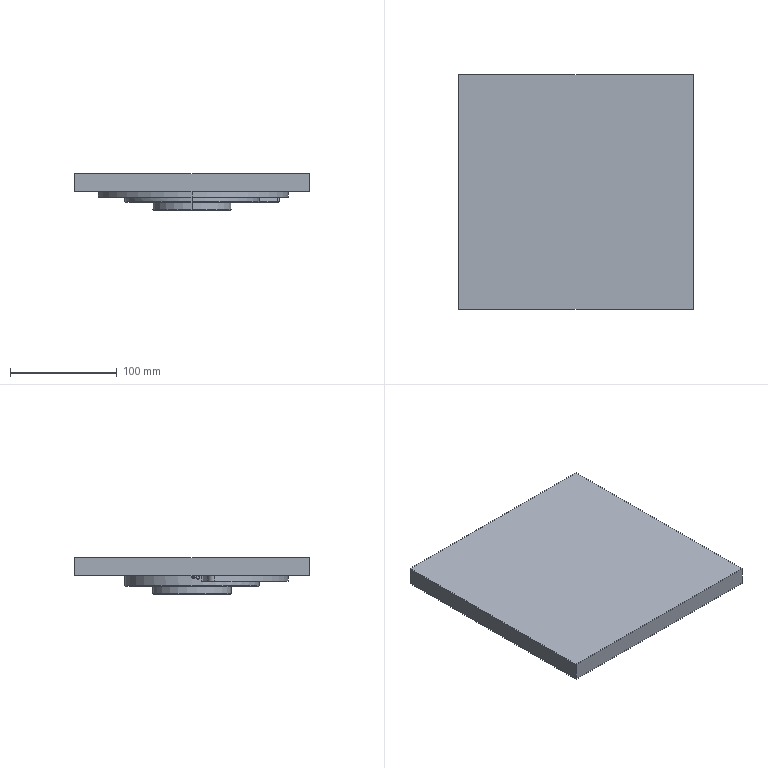NC program | NX | posted with a generic post | part box 220 x 220 x 34.5 mm
Lines 1 to 857 of 5610:
N10 G17 G21 G94 G90
(ADAPTIVE_MILLING_COPY_COPY , TOOL : D10)
N12 T03 M6
N14 G54
N16 G17 G0 G90 X77.604 Y4.579 S8000 M3
N18 G43 Z30. H3
N20 Z-4.5
N22 G94 G3 X77.604 Y4.579 Z-4.994 I3.735 J2.51 F1000.
N24 X77.604 Y4.579 Z-5.487 I3.735 J2.51
N26 X77.604 Y4.579 Z-5.981 I3.735 J2.51
N28 X77.604 Y4.579 Z-6.474 I3.735 J2.51
N30 X77.604 Y4.579 Z-6.968 I3.735 J2.51
N32 X77.604 Y4.579 Z-7.461 I3.735 J2.51
N34 X77.604 Y4.579 Z-7.955 I3.735 J2.51
N36 X77.604 Y4.579 Z-8.448 I3.735 J2.51
N38 X77.604 Y4.579 Z-8.942 I3.735 J2.51
N40 X77.604 Y4.579 Z-9.435 I3.735 J2.51
N42 X77.604 Y4.579 Z-9.929 I3.735 J2.51
N44 X77.604 Y4.579 Z-10.422 I3.735 J2.51
N46 X77.604 Y4.579 Z-10.916 I3.735 J2.51
N48 X77.604 Y4.579 Z-11.409 I3.735 J2.51
N50 X77.604 Y4.579 Z-11.903 I3.735 J2.51
N52 X76.839 Y7.09 Z-12.35 R-4.5
N54 X77.66 Y9.695 R-4.501 F3500.
N56 X82.637 Y2.294 R4.676
N58 X77.753 Y10.564 R-4.978
N60 X82.99 Y1.881 R5.196
N62 X77.662 Y11.175 R-5.477
N64 X83.422 Y1.484 R5.718
N66 X77.823 Y11.975 R-5.997
N68 X83.941 Y1.117 R6.258
N70 X77.688 Y12.541 R-6.537
N72 X84.559 Y0.793 R6.812
N74 X77.483 Y13.088 R-7.1
N76 X83.873 Y-0.126 R7.381
N78 X77.889 Y13.978 R-7.675
N80 X84.342 Y-0.592 R7.973
N82 X77.892 Y14.646 R-8.276
N84 X83.756 Y-1.428 R8.576
N86 X78.185 Y15.432 R-8.886
N88 X83.669 Y-2.101 R9.197
N90 X78.37 Y16.172 R-9.518
N92 X83.294 Y-2.846 R9.839
N94 X78.844 Y16.978 R-10.163
N96 X83.079 Y-3.549 R10.488
N98 X92.013 Y8.867 R10.816
N100 X79.62 Y17.804 R10.816
N102 X81.164 Y-4.346 R11.144
N104 X80.698 Y18.596 R-11.481
N106 X80.371 Y-4.984 R11.82
N108 X81.085 Y19.297 R-12.163
N110 X78.334 Y-5.339 R12.502
N112 X84.706 Y19.543 R12.843
N114 X69.985 Y0.098 R13.156
N116 X92.331 Y-0.932 R13.367
N118 X94.815 Y5.085 R13.688
N120 X94.218 Y11.135 R35.729
N122 X84.437 Y20.378 R13.14
N124 X67.552 Y8.958 R13.88
N126 X68.166 Y2.887 R147.626
N128 X74.962 Y-5.635 R12.919
N130 X94.942 Y2.514 R14.21
N132 G1 X94.812 Y5.136
N134 X94.408 Y10.154
N136 G3 X93.955 Y13.241 R19.214
N138 X89.674 Y18.793 R11.441
N140 X67.243 Y11.02 R14.568
N142 X67.535 Y9.129 R13.812
N144 G1 X67.56 Y8.88
N146 G3 X68.1 Y8.383 R0.554
N148 G1 X70.083 Y8.641 Z-12.25
N150 X91.724 Y11.521
N152 X93.706 Y11.786 Z-12.35
N154 G3 X94.152 Y12.389 R0.553
N156 X93.635 Y15.102 R9.567
N158 X88.948 Y20.151 R11.318
N160 X66.997 Y12.595 R15.277
N162 G1 X66.974 Y12.472
N164 X66.969 Y12.387
N166 X67.248 Y10.786
N168 G3 X67.828 Y10.331 R0.554
N170 G1 X69.813 Y10.576 Z-12.25
N172 X91.526 Y13.265
N174 X93.51 Y13.514 Z-12.35
N176 G3 X93.932 Y14.148 R0.553
N178 X93.286 Y16.681 R9.094
N180 X88.91 Y21.021 R10.806
N182 X66.842 Y14.109 R15.946
N184 G1 X66.796 Y13.993
N186 X66.757 Y13.874
N188 X66.741 Y13.75
N190 X66.739 Y13.708
N192 X66.975 Y12.354
N194 G3 X67.555 Y11.899 R0.554
N196 G1 X69.541 Y12.137 Z-12.25
N198 X91.273 Y14.75
N200 X93.258 Y14.993 Z-12.35
N202 G3 X93.665 Y15.624 R0.553
N204 X92.737 Y18.446 R6.65
N206 X87.147 Y22.693 R11.904
N208 X66.759 Y15.566 R16.65
N210 X66.653 Y14.203 R1.411
N212 G1 X66.76 Y13.587
N214 G3 X67.34 Y13.133 R0.554
N216 G1 X69.326 Y13.371 Z-12.25
N218 X91.05 Y15.98
N220 X93.035 Y16.223 Z-12.35
N222 G3 X93.442 Y16.854 R0.553
N224 X91.293 Y20.959 R6.144
N226 X82.546 Y24.546 R14.666
N228 X66.733 Y16.974 R17.347
N230 X66.254 Y15.782 R2.529
N232 G1 X66.53 Y14.691
N234 G3 X67.142 Y14.281 R0.554
N236 G1 X69.128 Y14.517 Z-12.25
N238 X90.851 Y17.091
N240 X92.836 Y17.33 Z-12.35
N242 G3 X93.242 Y17.962 R0.553
N244 X91.196 Y21.843 R5.78
N246 X83.037 Y25.286 R14.46
N248 X66.683 Y18.235 R17.99
N250 X66.01 Y16.748 R2.99
N252 G1 X66.255 Y15.778
N254 G3 X66.885 Y15.371 R0.555
N256 G1 X68.872 Y15.597 Z-12.25
N258 X90.672 Y18.083
N260 X92.658 Y18.314 Z-12.35
N262 G3 X93.064 Y18.946 R0.553
N264 X90.875 Y22.904 R5.754
N266 X82.991 Y26.077 R14.51
N268 X66.72 Y19.544 R18.632
N270 X65.767 Y17.806 R4.756
N272 G1 X65.769 Y17.698
N274 X66.015 Y16.728
N276 G3 X66.643 Y16.321 R0.555
N278 G1 X68.629 Y16.558 Z-12.25
N280 X90.475 Y19.167
N282 X92.46 Y19.41 Z-12.35
N284 G3 X92.85 Y20.074 R0.553
N286 X91.839 Y22.602 R6.034
N288 X86.831 Y25.985 R10.861
N290 X71.491 Y24.508 R18.847
N292 X66.104 Y19.934 R16.021
N294 X65.532 Y18.637 R2.549
N296 G1 X65.777 Y17.668
N298 G3 X66.403 Y17.26 R0.554
N300 G1 X68.388 Y17.509 Z-12.25
N302 X90.222 Y20.25
N304 X92.205 Y20.506 Z-12.35
N306 G3 X92.579 Y21.165 R0.553
N308 X90.173 Y24.969 R5.71
N310 X82.254 Y27.726 R14.879
N312 X66.887 Y22.068 R19.896
N314 X65.296 Y19.704 R6.399
N316 X65.544 Y18.59 R4.388
N318 X66.169 Y18.183 R0.554
N320 G1 X68.153 Y18.435 Z-12.25
N322 X89.981 Y21.217
N324 X91.964 Y21.477 Z-12.35
N326 G3 X92.337 Y22.136 R0.553
N328 X89.993 Y25.832 R5.517
N330 X82.554 Y28.495 R14.604
N332 X66.734 Y23.02 R20.354
N334 X65.046 Y20.573 R6.607
N336 G1 X65.023 Y20.45
N338 X65.025 Y20.325
N340 X65.03 Y20.273
N342 X65.308 Y19.443
N344 G3 X65.943 Y19.078 R0.557
N346 G1 X67.926 Y19.337 Z-12.25
N348 X89.742 Y22.182
N350 X91.724 Y22.448 Z-12.35
N352 G3 X92.096 Y23.106 R0.553
N354 X89.901 Y26.614 R5.308
N356 X82.721 Y29.267 R14.208
N358 X66.672 Y24.049 R20.802
N360 X64.791 Y21.435 R7.048
N362 G1 X64.758 Y21.315
N364 X64.749 Y21.19
N366 X64.761 Y21.076
N368 X65.039 Y20.247
N370 G3 X65.717 Y19.888 R0.566
N372 G1 X67.698 Y20.159 Z-12.25
N374 X89.504 Y23.14
N376 X91.484 Y23.419 Z-12.35
N378 G3 X91.855 Y24.077 R0.553
N380 X89.603 Y27.545 R5.259
N382 X82.508 Y30.081 R14.321
N384 X66.613 Y25.065 R21.264
N386 X64.532 Y22.292 R7.52
N388 G1 X64.486 Y21.895
N390 X64.764 Y21.066
N392 G3 X65.441 Y20.707 R0.566
N394 G1 X67.423 Y20.979 Z-12.25
N396 X89.293 Y23.988
N398 X91.273 Y24.268 Z-12.35
N400 G3 X91.643 Y24.926 R0.553
N402 X89.58 Y28.257 R5.042
N404 X82.89 Y30.826 R13.722
N406 X66.45 Y25.975 R21.585
N408 X64.267 Y23.124 R7.674
N410 X64.213 Y22.709 R2.847
N412 G1 X64.491 Y21.879
N414 G3 X65.165 Y21.52 R0.562
N416 G1 X67.143 Y21.813 Z-12.25
N418 X89.03 Y25.048
N420 X91.007 Y25.349 Z-12.35
N422 G3 X91.357 Y26.038 R0.553
N424 X88.845 Y29.481 R5.525
N426 X81.527 Y31.751 R14.884
N428 X66.478 Y27.041 R22.046
N430 X64.044 Y24.071 R8.357
N432 X63.942 Y23.518 R1.482
N434 G1 X64.22 Y22.689
N436 G3 X64.893 Y22.33 R0.562
N438 G1 X66.871 Y22.624 Z-12.25
N440 X88.775 Y25.882
N442 X89.765 Y26.023 Z-12.3
N444 X90.751 Y26.186 Z-12.35
N446 G3 X91.092 Y26.872 R0.553
N448 X88.604 Y30.327 R5.417
N450 X81.4 Y32.554 R14.727
N452 X66.313 Y27.935 R22.335
N454 X63.775 Y24.891 R8.567
N456 X63.754 Y24.08 R0.865
N458 G1 X63.952 Y23.487
N460 G3 X64.623 Y23.128 R0.56
N462 G1 X66.599 Y23.435 Z-12.25
N464 X88.475 Y26.824
N466 X89.464 Y26.971 Z-12.3
N468 X90.449 Y27.14 Z-12.35
N470 G3 X90.788 Y27.824 R0.553
N472 X88.356 Y31.17 R5.273
N474 X81.393 Y33.349 R14.506
N476 X66.049 Y28.748 R22.524
N478 X63.458 Y25.593 R8.321
N480 X63.375 Y24.979 R1.192
N482 G1 X63.715 Y24.173
N484 G3 X64.377 Y23.854 R0.562
N486 G1 X66.35 Y24.178 Z-12.25
N488 X88.178 Y27.76
N490 X89.165 Y27.917 Z-12.3
N492 X90.149 Y28.094 Z-12.35
N494 G3 X90.484 Y28.777 R0.553
N496 X88.101 Y32.01 R5.158
N498 X80.881 Y34.178 R14.597
N500 X65.783 Y29.556 R22.715
N502 X63.182 Y26.407 R8.547
N504 X63.067 Y25.71 R1.319
N506 G1 X63.407 Y24.904
N508 G3 X64.126 Y24.595 R0.589
N510 G1 X66.098 Y24.926 Z-12.25
N512 X87.914 Y28.587
N514 X88.901 Y28.748 Z-12.3
N516 X89.884 Y28.928 Z-12.35
N518 G3 X90.219 Y29.611 R0.553
N520 X87.842 Y32.846 R5.102
N522 X80.99 Y34.964 R14.318
N524 X65.612 Y30.441 R22.876
N526 X62.899 Y27.222 R8.959
N528 X62.755 Y26.45 R1.505
N530 G1 X63.095 Y25.644
N532 G3 X63.817 Y25.337 R0.591
N534 G1 X65.789 Y25.674 Z-12.25
N536 X87.65 Y29.415
N538 X88.637 Y29.58 Z-12.3
N540 X89.62 Y29.762 Z-12.35
N542 G3 X89.953 Y30.445 R0.553
N544 X87.581 Y33.681 R5.069
N546 X80.846 Y35.768 R14.193
N548 X65.44 Y31.323 R23.04
N550 X62.567 Y27.919 R9.131
N552 X62.444 Y27.188 R1.317
N554 G1 X62.784 Y26.382
N556 G3 X63.504 Y26.075 R0.588
N558 G1 X65.475 Y26.419 Z-12.25
N560 X87.387 Y30.243
N562 X88.372 Y30.411 Z-12.3
N564 X89.355 Y30.596 Z-12.35
N566 G3 X89.687 Y31.278 R0.553
N568 X87.075 Y34.664 R5.35
N570 X79.917 Y36.621 R14.9
N572 X65.241 Y32.18 R23.194
N574 X62.263 Y28.704 R9.32
N576 X62.125 Y27.943 R1.473
N578 G1 X62.465 Y27.137
N580 G3 X63.18 Y26.83 R0.58
N582 G1 X65.147 Y27.196 Z-12.25
N584 X87.032 Y31.272
N586 X88.943 Y31.631 Z-12.347
N588 X88.996 Y31.649 Z-12.35
N590 G3 X89.299 Y32.359 R0.553
N592 X86.676 Y35.563 R5.377
N594 X79.619 Y37.433 R15.012
N596 X64.947 Y32.966 R23.354
N598 X61.962 Y29.494 R9.461
N600 X61.809 Y28.694 R1.487
N602 G1 X62.149 Y27.887
N604 G3 X62.86 Y27.58 R0.576
N606 G1 X64.824 Y27.961 Z-12.25
N608 X86.673 Y32.19
N610 X88.581 Y32.563 Z-12.347
N612 X88.633 Y32.581 Z-12.35
N614 G3 X88.935 Y33.29 R0.553
N616 X86.377 Y36.392 R5.257
N618 X79.316 Y38.243 R14.909
N620 X64.75 Y33.827 R23.46
N622 X61.71 Y30.395 R10.117
N624 X61.498 Y29.325 R1.6
N626 G1 X61.744 Y28.845
N628 X61.753 Y28.826
N630 X61.85 Y28.595
N632 G3 X62.56 Y28.288 R0.574
N634 G1 X64.522 Y28.677 Z-12.25
N636 X86.357 Y32.998
N638 X88.264 Y33.378 Z-12.347
N640 X88.316 Y33.397 Z-12.35
N642 G3 X88.616 Y34.105 R0.553
N644 X85.967 Y37.281 R5.262
N646 X78.76 Y39.059 R15.101
N648 X64.55 Y34.684 R23.593
N650 X61.354 Y31.066 R10.085
N652 X61.153 Y29.996 R1.652
N654 G1 X61.553 Y29.217
N656 G3 X62.275 Y28.956 R0.591
N658 G1 X64.232 Y29.364 Z-12.25
N660 X86. Y33.91
N662 X87.904 Y34.311 Z-12.347
N664 X87.955 Y34.33 Z-12.35
N666 G3 X88.251 Y35.036 R0.553
N668 X85.659 Y38.103 R5.153
N670 X78.7 Y39.86 R14.853
N672 X64.146 Y35.391 R23.62
N674 X60.991 Y31.739 R9.969
N676 X60.8 Y30.683 R1.698
N678 G1 X61.2 Y29.904
N680 G3 X61.804 Y29.618 R0.555
N682 G1 X61.963 Y29.652
N684 X63.919 Y30.07 Z-12.25
N686 X85.685 Y34.717
N688 X87.587 Y35.126 Z-12.347
N690 X87.638 Y35.145 Z-12.35
N692 G3 X87.932 Y35.85 R0.553
N694 X85.347 Y38.924 R5.144
N696 X78.26 Y40.669 R14.839
N698 X63.839 Y36.168 R23.661
N700 X60.623 Y32.407 R10.02
N702 X60.441 Y31.38 R1.71
N704 G1 X60.841 Y30.602
N706 G3 X61.447 Y30.316 R0.555
N708 G1 X61.602 Y30.35
N710 X63.557 Y30.775 Z-12.25
N712 X85.368 Y35.525
N714 X86.347 Y35.731 Z-12.3
N716 X87.32 Y35.96 Z-12.35
N718 G3 X87.613 Y36.665 R0.553
N720 X85.015 Y39.757 R5.17
N722 X78.046 Y41.473 R14.831
N724 X63.512 Y36.931 R23.71
N726 X60.289 Y33.173 R10.282
N728 X60.084 Y32.076 R1.754
N730 G1 X60.484 Y31.298
N732 G3 X61.094 Y31.013 R0.555
N734 G1 X61.24 Y31.046
N736 X63.19 Y31.488 Z-12.25
N738 X85.015 Y36.428
N740 X86.909 Y36.86 Z-12.347
N742 X86.962 Y36.881 Z-12.35
N744 G3 X87.231 Y37.615 R0.553
N746 X84.241 Y40.817 R5.627
N748 X76.958 Y42.281 R15.76
N750 X63.086 Y37.622 R23.684
N752 X59.903 Y33.831 R10.194
N754 X59.72 Y32.784 R1.729
N756 G1 X60.12 Y32.006
N758 G3 X60.735 Y31.721 R0.555
N760 G1 X60.871 Y31.753
N762 X62.819 Y32.21 Z-12.25
N764 X84.601 Y37.321
N766 X86.49 Y37.768 Z-12.347
N768 X86.544 Y37.79 Z-12.35
N770 G3 X86.807 Y38.52 R0.553
N772 X83.897 Y41.632 R5.473
N774 X76.612 Y43.084 R15.641
N776 X62.753 Y38.384 R23.787
N778 X59.561 Y34.598 R10.468
N780 X59.364 Y33.467 R1.714
N782 G1 X59.389 Y33.425
N784 X59.4 Y33.407
N786 X59.743 Y32.74
N788 G3 X60.361 Y32.457 R0.554
N790 G1 X60.49 Y32.488
N792 X62.434 Y32.958 Z-12.25
N794 X84.182 Y38.215
N796 X86.069 Y38.674 Z-12.347
N798 X86.122 Y38.697 Z-12.35
N800 G3 X86.383 Y39.426 R0.553
N802 X83.55 Y42.444 R5.348
N804 X76.264 Y43.882 R15.467
N806 X62.417 Y39.145 R23.759
N808 X59.168 Y35.248 R10.498
N810 X58.997 Y34.065 R1.734
N812 G1 X59.389 Y33.426
N814 G3 X60.116 Y33.211 R0.597
N816 G1 X62.056 Y33.695 Z-12.25
N818 X83.765 Y39.108
N820 X85.649 Y39.581 Z-12.347
N822 X85.702 Y39.604 Z-12.35
N824 G3 X85.959 Y40.331 R0.553
N826 X83.199 Y43.255 R5.26
N828 X76.036 Y44.682 R15.291
N830 X61.881 Y39.749 R23.689
N832 X58.771 Y35.897 R10.273
N834 X58.609 Y34.698 R1.769
N836 G1 X59.001 Y34.059
N838 G3 X59.606 Y33.814 R0.555
N840 G1 X59.78 Y33.858
N842 X61.718 Y34.353 Z-12.25
N844 X83.398 Y39.891
N846 X85.28 Y40.375 Z-12.347
N848 X85.333 Y40.397 Z-12.35
N850 G3 X85.588 Y41.124 R0.553
N852 X82.732 Y44.117 R5.306
N854 X75.555 Y45.476 R15.367
N856 X61.633 Y40.588 R23.8
N858 X58.369 Y36.548 R10.417
N860 X58.209 Y35.349 R1.791
N862 G1 X58.667 Y34.603
N864 G3 X59.277 Y34.359 R0.555
N866 G1 X59.465 Y34.409
N868 X61.398 Y34.923 Z-12.25
N870 X83.035 Y40.667
N872 X84.913 Y41.169 Z-12.347
N874 X84.964 Y41.191 Z-12.35
N876 G3 X85.217 Y41.916 R0.553
N878 X82.376 Y44.923 R5.263
N880 X75.323 Y46.273 R15.173
N882 X61.191 Y41.27 R23.818
N884 X57.96 Y37.202 R10.482
N886 X57.805 Y36.009 R1.81
N888 G1 X58.262 Y35.263
N890 G3 X58.877 Y35.02 R0.555
N892 G1 X59.054 Y35.069
N894 X60.982 Y35.6 Z-12.25
N896 X82.618 Y41.557
N898 X84.493 Y42.076 Z-12.347
N900 X84.543 Y42.098 Z-12.35
N902 G3 X84.793 Y42.822 R0.553
N904 X81.642 Y45.899 R5.644
N906 X74.175 Y47.033 R16.044
N908 X60.813 Y42.002 R23.765
N910 X57.534 Y37.817 R10.46
N912 X57.396 Y36.674 R1.851
N914 G1 X57.854 Y35.929
N916 G3 X58.475 Y35.688 R0.555
N918 G1 X58.637 Y35.735
N920 X60.558 Y36.29 Z-12.25
N922 X82.117 Y42.52
N924 X83.981 Y43.062 Z-12.347
N926 X84.034 Y43.087 Z-12.35
N928 G3 X84.254 Y43.836 R0.553
N930 X81.256 Y46.698 R5.495
N932 X74.038 Y47.833 R15.672
N934 X60.441 Y42.745 R23.866
N936 X57.154 Y38.564 R10.767
N938 X56.988 Y37.339 R1.873
N940 G1 X57.446 Y36.594
N942 G3 X58.072 Y36.354 R0.555
N944 G1 X58.224 Y36.399
N946 X60.14 Y36.971 Z-12.25
N948 X81.643 Y43.382
N950 X83.503 Y43.94 Z-12.347
N952 X83.555 Y43.965 Z-12.35
N954 G3 X83.772 Y44.712 R0.553
N956 X80.635 Y47.596 R5.503
N958 X73.021 Y48.577 R16.315
N960 X59.874 Y43.323 R23.747
N962 X56.723 Y39.191 R10.615
N964 X56.596 Y37.953 R1.732
N966 G1 X56.696 Y37.815
N968 X56.707 Y37.797
N970 X57.034 Y37.265
N972 G3 X57.662 Y37.026 R0.555
N974 G1 X57.81 Y37.07
N976 X59.724 Y37.649 Z-12.25
N978 X81.225 Y44.143
N980 X83.083 Y44.707 Z-12.347
N982 X83.135 Y44.733 Z-12.35
N984 G3 X83.351 Y45.479 R0.553
N986 X80.239 Y48.386 R5.438
N988 X72.875 Y49.377 R15.876
N990 X59.589 Y44.144 R23.862
N992 X56.33 Y39.936 R11.04
N994 X56.174 Y38.537 R1.988
N996 G1 X56.613 Y37.929
N998 G3 X57.222 Y37.726 R0.555
N1000 G1 X57.375 Y37.773
N1002 X59.286 Y38.364 Z-12.25
N1004 X80.75 Y45.008
N1006 X82.604 Y45.585 Z-12.347
N1008 X82.657 Y45.611 Z-12.35
N1010 G3 X82.869 Y46.355 R0.553
N1012 X79.838 Y49.175 R5.366
N1014 X72.474 Y50.155 R15.673
N1016 X59.016 Y44.716 R23.768
N1018 X55.853 Y40.441 R10.67
N1020 X55.743 Y39.132 R1.908
N1022 G1 X56.183 Y38.524
N1024 G3 X56.797 Y38.323 R0.555
N1026 G1 X56.993 Y38.386
N1028 X58.897 Y38.998 Z-12.25
N1030 X80.279 Y45.866
N1032 X82.127 Y46.463 Z-12.347
N1034 X82.178 Y46.489 Z-12.35
N1036 G3 X82.387 Y47.231 R0.553
N1038 X79.55 Y49.912 R5.197
N1040 X72.446 Y50.961 R15.17
N1042 X58.63 Y45.453 R23.849
N1044 X55.449 Y41.187 R11.049
N1046 X55.261 Y39.842 R2.739
N1048 G1 X55.305 Y39.739
N1050 X55.744 Y39.131
N1052 G3 X56.361 Y38.931 R0.555
N1054 G1 X56.568 Y38.998
N1056 X58.469 Y39.621 Z-12.25
N1058 X79.862 Y46.624
N1060 X81.708 Y47.231 Z-12.347
N1062 X81.759 Y47.257 Z-12.35
N1064 G3 X81.965 Y47.998 R0.553
N1066 X78.654 Y50.899 R5.622
N1068 X71.013 Y51.644 R16.309
N1070 X58.215 Y46.168 R23.85
N1072 X54.991 Y41.782 R11.04
N1074 X54.853 Y40.364 R2.083
N1076 G1 X55.366 Y39.655
N1078 G3 X55.992 Y39.458 R0.555
N1080 G1 X56.177 Y39.522
N1082 X58.066 Y40.178 Z-12.25
N1084 X79.317 Y47.552
N1086 X81.148 Y48.191 Z-12.347
N1088 X81.201 Y48.219 Z-12.35
N1090 G3 X81.376 Y48.983 R0.553
N1092 X78.105 Y51.723 R5.655
N1094 X70.706 Y52.426 R16.154
N1096 X57.711 Y46.803 R23.86
N1098 X54.528 Y42.386 R11.115
N1100 X54.4 Y40.991 R2.119
N1102 G1 X54.912 Y40.282
N1104 G3 X55.543 Y40.086 R0.555
N1106 G1 X55.717 Y40.148
N1108 X57.601 Y40.821 Z-12.25
N1110 X78.788 Y48.381
N1112 X80.615 Y49.036 Z-12.347
N1114 X80.667 Y49.065 Z-12.35
N1116 G3 X80.839 Y49.827 R0.553
N1118 X77.553 Y52.544 R5.563
N1120 X70.023 Y53.162 R16.284
N1122 X57.112 Y47.352 R23.767
N1124 X54.025 Y42.872 R10.838
N1126 X53.945 Y41.621 R1.933
N1128 G1 X54.457 Y40.912
N1130 G3 X55.092 Y40.717 R0.555
N1132 G1 X55.257 Y40.778
N1134 X57.134 Y41.466 Z-12.25
N1136 X78.26 Y49.21
N1138 X80.081 Y49.881 Z-12.347
N1140 X80.132 Y49.91 Z-12.35
N1142 G3 X80.301 Y50.67 R0.553
N1144 X77.111 Y53.312 R5.436
N1146 X69.706 Y53.94 R15.945
N1148 X56.599 Y47.983 R23.82
N1150 X53.59 Y43.593 R11.07
N1152 X53.478 Y42.248 R2.129
N1154 G1 X53.508 Y42.19
N1156 X53.678 Y41.989
N1158 X53.691 Y41.972
N1160 X53.984 Y41.567
N1162 G3 X54.623 Y41.374 R0.555
N1164 G1 X54.778 Y41.432
N1166 X56.651 Y42.135 Z-12.25
N1168 X77.73 Y50.041
N1170 X79.547 Y50.726 Z-12.347
N1172 X79.598 Y50.755 Z-12.35
N1174 G3 X79.764 Y51.513 R0.553
N1176 X76.547 Y54.122 R5.395
N1178 X69.014 Y54.665 R16.047
N1180 X56.085 Y48.609 R23.745
N1182 X53.114 Y44.193 R11.081
N1184 X52.995 Y42.842 R2.647
N1186 G1 X53.053 Y42.728
N1188 X53.537 Y42.156
N1190 G3 X54.152 Y41.996 R0.555
N1192 G1 X54.322 Y42.061
N1194 X56.192 Y42.771 Z-12.25
N1196 X77.265 Y50.773
N1198 X79.079 Y51.465 Z-12.347
N1200 X79.13 Y51.494 Z-12.35
N1202 G3 X79.293 Y52.251 R0.553
N1204 X76.1 Y54.887 R5.381
N1206 X68.939 Y55.47 R15.574
N1208 X55.57 Y49.232 R23.737
N1210 X52.633 Y44.793 R11.027
N1212 X52.558 Y43.325 R2.203
N1214 G1 X52.571 Y43.299
N1216 X53.055 Y42.726
N1218 G3 X53.676 Y42.569 R0.555
N1220 G1 X53.888 Y42.652
N1222 X55.75 Y43.381 Z-12.25
N1224 X76.738 Y51.6
N1226 X78.545 Y52.311 Z-12.347
N1228 X78.595 Y52.34 Z-12.35
N1230 G3 X78.756 Y53.094 R0.553
N1232 X75.385 Y55.739 R5.558
N1234 X68.088 Y56.169 R15.943
N1236 X55.028 Y49.834 R23.777
N1238 X52.14 Y45.364 R11.098
N1240 X52.075 Y43.894 R2.222
N1242 G1 X52.087 Y43.872
N1244 X52.652 Y43.204
N1246 G3 X53.282 Y43.05 R0.555
N1248 G1 X53.484 Y43.133
N1250 X55.332 Y43.897 Z-12.25
N1252 X76.141 Y52.493
N1254 X77.932 Y53.237 Z-12.347
N1256 X77.983 Y53.269 Z-12.35
N1258 G3 X78.111 Y54.044 R0.553
N1260 X74.67 Y56.571 R5.711
N1262 X66.996 Y56.815 R16.456
N1264 X54.404 Y50.347 R23.63
N1266 X51.613 Y45.819 R10.735
N1268 X51.593 Y44.456 R1.98
N1270 G1 X52.158 Y43.788
N1272 G3 X52.793 Y43.636 R0.555
N1274 G1 X52.983 Y43.717
N1276 X54.825 Y44.497 Z-12.25
N1278 X75.56 Y53.286
N1280 X77.345 Y54.046 Z-12.347
N1282 X77.396 Y54.078 Z-12.35
N1284 G3 X77.52 Y54.851 R0.553
N1286 X74.189 Y57.322 R5.561
N1288 X66.762 Y57.599 R16.056
N1290 X53.948 Y51.038 R23.769
N1292 X51.11 Y46.395 R10.907
N1294 X51.04 Y45.16 R2.912
N1296 X51.663 Y44.373 R15.811
N1298 X52.303 Y44.224 R0.555
N1300 G1 X52.482 Y44.302
N1302 X54.316 Y45.099 Z-12.25
N1304 X74.98 Y54.078
N1306 X76.758 Y54.855 Z-12.347
N1308 X76.808 Y54.887 Z-12.35
N1310 G3 X76.929 Y55.657 R0.553
N1312 X73.583 Y58.104 R5.498
N1314 X66.154 Y58.314 R16.017
N1316 X53.399 Y51.637 R23.767
N1318 X50.604 Y46.968 R10.978
N1320 X50.603 Y45.629 R1.95
N1322 G1 X51.167 Y44.96
N1324 G3 X51.811 Y44.813 R0.555
N1326 G1 X51.98 Y44.888
N1328 X53.807 Y45.701 Z-12.25
N1330 X74.399 Y54.871
N1332 X76.171 Y55.664 Z-12.347
N1334 X76.22 Y55.696 Z-12.35
N1336 G3 X76.338 Y56.464 R0.553
N1338 X72.974 Y58.883 R5.45
N1340 X65.421 Y59.001 R16.154
N1342 X52.85 Y52.232 R23.702
N1344 X50.091 Y47.54 R11.007
N1346 X50.1 Y46.193 R1.981
N1348 G1 X50.122 Y46.159
N1350 X50.354 Y45.923
N1352 X50.368 Y45.907
N1354 X50.61 Y45.62
N1356 G3 X51.257 Y45.474 R0.555
N1358 G1 X51.418 Y45.547
N1360 X53.241 Y46.371 Z-12.25
N1362 X73.815 Y55.669
N1364 X75.582 Y56.472 Z-12.347
N1366 X75.631 Y56.504 Z-12.35
N1368 G3 X75.747 Y57.271 R0.553
N1370 X72.479 Y59.618 R5.353
N1372 X65.173 Y59.778 R15.769
N1374 X52.296 Y52.823 R23.772
N1376 X49.575 Y48.109 R11.036
N1378 X49.569 Y46.754 R2.486
N1380 G1 X49.625 Y46.663
N1382 X50.151 Y46.128
N1384 G3 X50.773 Y46.014 R0.555
N1386 G1 X50.951 Y46.096
N1388 X52.769 Y46.931 Z-12.25
N1390 X73.305 Y56.366
N1392 X75.068 Y57.179 Z-12.347
N1394 X75.117 Y57.212 Z-12.35
N1396 G3 X75.23 Y57.977 R0.553
N1398 X71.836 Y60.393 R5.481
N1400 X64.406 Y60.449 R15.88
N1402 X51.637 Y53.299 R23.78
N1404 X49.049 Y48.651 R10.878
N1406 X49.045 Y47.294 R2.738
N1408 G1 X49.11 Y47.187
N1410 X49.636 Y46.652
N1412 G3 X50.265 Y46.541 R0.555
N1414 G1 X50.479 Y46.643
N1416 X52.284 Y47.505 Z-12.25
N1418 X72.652 Y57.229
N1420 X74.4 Y58.068 Z-12.347
N1422 X74.45 Y58.103 Z-12.35
N1424 G3 X74.532 Y58.888 R0.552
N1426 X70.832 Y61.25 R5.827
N1428 X62.913 Y60.942 R16.868
N1430 X51.23 Y54.059 R23.746
N1432 X48.543 Y49.322 R11.314
N1434 X48.512 Y47.84 R3.067
N1436 X49.194 Y47.102 R13.595
N1438 X49.83 Y46.994 R0.555
N1440 G1 X50.035 Y47.096
N1442 X51.827 Y47.983 Z-12.25
N1444 X72.028 Y57.975
N1446 X73.765 Y58.838 Z-12.347
N1448 X73.814 Y58.874 Z-12.35
N1450 G3 X73.89 Y59.655 R0.553
N1452 X70.182 Y62. R5.771
N1454 X62.266 Y61.619 R16.831
N1456 X50.487 Y54.437 R23.598
N1458 X47.982 Y49.742 R10.972
N1460 X47.979 Y48.382 R2.997
N1462 X48.661 Y47.643 R12.175
N1464 X49.302 Y47.538 R0.555
N1466 G1 X49.495 Y47.636
N1468 X51.279 Y48.54 Z-12.25
N1470 X71.398 Y58.728
N1472 X73.127 Y59.608 Z-12.347
N1474 X73.175 Y59.643 Z-12.35
N1476 G3 X73.248 Y60.421 R0.553
N1478 X69.529 Y62.743 R5.699
N1480 X61.859 Y62.357 R16.642
N1482 X50.065 Y55.192 R23.791
N1484 X47.438 Y50.284 R11.295
N1486 X47.443 Y48.925 R2.96
N1488 X48.124 Y48.19 R23.555
N1490 X48.769 Y48.087 R0.555
N1492 G1 X48.951 Y48.181
N1494 X50.727 Y49.101 Z-12.25
N1496 X70.767 Y59.482
N1498 X72.489 Y60.377 Z-12.347
N1500 X72.536 Y60.412 Z-12.35
N1502 G3 X72.606 Y61.188 R0.553
N1504 X68.994 Y63.452 R5.547
N1506 X61.568 Y63.121 R16.179
N1508 X49.478 Y55.754 R23.807
N1510 X46.89 Y50.824 R11.389
N1512 X46.906 Y49.465 R2.805
N1514 G1 X46.968 Y49.365
N1516 X47.581 Y48.742
N1518 G3 X48.231 Y48.641 R0.555
N1520 G1 X48.402 Y48.732
N1522 X50.17 Y49.667 Z-12.25
N1524 X70.136 Y60.235
N1526 X71.85 Y61.146 Z-12.347
N1528 X71.897 Y61.182 Z-12.35
N1530 G3 X71.964 Y61.955 R0.553
N1532 X68.457 Y64.161 R5.436
N1534 X61.034 Y63.822 R15.979
N1536 X48.889 Y56.313 R23.82
N1538 X46.339 Y51.364 R11.423
N1540 X46.418 Y49.895 R2.215
N1542 G1 X46.453 Y49.846
N1544 X46.742 Y49.594
N1546 X46.757 Y49.58
N1548 X47.02 Y49.312
N1550 G3 X47.673 Y49.214 R0.555
N1552 G1 X47.835 Y49.301
N1554 X49.595 Y50.251 Z-12.25
N1556 X69.504 Y60.991
N1558 X71.212 Y61.915 Z-12.347
N1560 X71.258 Y61.951 Z-12.35
N1562 G3 X71.322 Y62.722 R0.553
N1564 X67.767 Y64.896 R5.499
N1566 X60.227 Y64.443 R16.117
N1568 X48.2 Y56.75 R23.765
N1570 X45.778 Y51.873 R11.298
N1572 X45.859 Y50.397 R2.623
N1574 G1 X45.922 Y50.31
N1576 X46.487 Y49.817
N1578 G3 X47.114 Y49.749 R0.555
N1580 G1 X47.293 Y49.847
N1582 X49.045 Y50.812 Z-12.25
N1584 X68.875 Y61.728
N1586 X70.572 Y62.666 Z-12.347
N1588 X70.62 Y62.704 Z-12.35
N1590 G3 X70.653 Y63.495 R0.552
N1592 X66.712 Y65.687 R5.939
N1594 X59.065 Y64.952 R16.806
N1596 X47.592 Y57.286 R23.725
N1598 X45.197 Y52.263 R11.058
N1600 X45.288 Y50.907 R2.937
N1602 X45.93 Y50.303 R11.068
N1604 X46.565 Y50.239 R0.555
N1606 G1 X46.776 Y50.36
N1608 X48.514 Y51.35 Z-12.25
N1610 X68.118 Y62.522
N1612 X69.802 Y63.485 Z-12.347
N1614 X69.849 Y63.523 Z-12.35
N1616 G3 X69.876 Y64.309 R0.553
N1618 X66.141 Y66.375 R5.686
N1620 X58.379 Y65.591 R16.659
N1622 X46.905 Y57.716 R23.628
N1624 X44.63 Y52.772 R10.906
N1626 X44.716 Y51.414 R3.124
N1628 X45.457 Y50.717 R5.915
N1630 X46.098 Y50.657 R0.555
N1632 G1 X46.298 Y50.775
N1634 X48.022 Y51.789 Z-12.25
N1636 X67.447 Y63.226
N1638 X69.117 Y64.213 Z-12.347
N1640 X69.163 Y64.251 Z-12.35
N1642 G3 X69.186 Y65.033 R0.553
N1644 X65.442 Y67.076 R5.623
N1646 X57.806 Y66.264 R16.473
N1648 X46.363 Y58.342 R23.694
N1650 X44.055 Y53.277 R11.193
N1652 X44.212 Y51.814 R2.258
N1654 G1 X44.229 Y51.79
N1656 X44.888 Y51.214
N1658 G3 X45.533 Y51.157 R0.555
N1660 G1 X45.722 Y51.27
N1662 X47.435 Y52.301 Z-12.25
N1664 X66.77 Y63.936
N1666 X68.431 Y64.939 Z-12.347
N1668 X68.476 Y64.978 Z-12.35
N1670 G3 X68.496 Y65.757 R0.553
N1672 X64.739 Y67.773 R5.589
N1674 X57.229 Y66.932 R16.438
N1676 X45.744 Y58.862 R23.699
N1678 X43.475 Y53.78 R11.226
N1680 X43.635 Y52.317 R2.25
N1682 G1 X43.65 Y52.295
N1684 X44.309 Y51.72
N1686 G3 X44.959 Y51.665 R0.555
N1688 G1 X45.136 Y51.774
N1690 X46.84 Y52.821 Z-12.25
N1692 X66.092 Y64.647
N1694 X67.744 Y65.666 Z-12.347
N1696 X67.789 Y65.704 Z-12.35
N1698 G3 X67.806 Y66.48 R0.553
N1700 X64.158 Y68.445 R5.454
N1702 X56.652 Y67.597 R16.122
N1704 X45.047 Y59.281 R23.759
N1706 X42.891 Y54.281 R11.266
N1708 X43.058 Y52.819 R2.231
N1710 G1 X43.071 Y52.801
N1712 X43.73 Y52.226